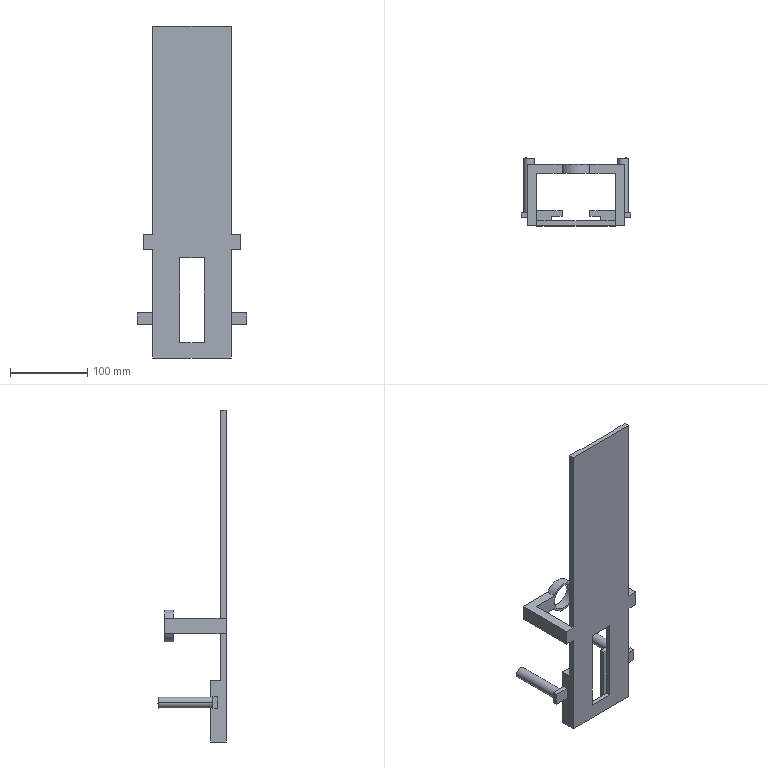Part | SolidWorks | features ICE 9, BossThin 2, MirrorPattern 2, Extrusion 1, Helix 1, RefPoint 1, Sweep 1 | 1 solid | 74 faces | box 142 x 88.365 x 430 mm | volume 380950 mm3 | plane 58 | cylinder 12 | spline 4 | commonest cylinder face diameters 12 x4 14 x4 35 x2 41 x2